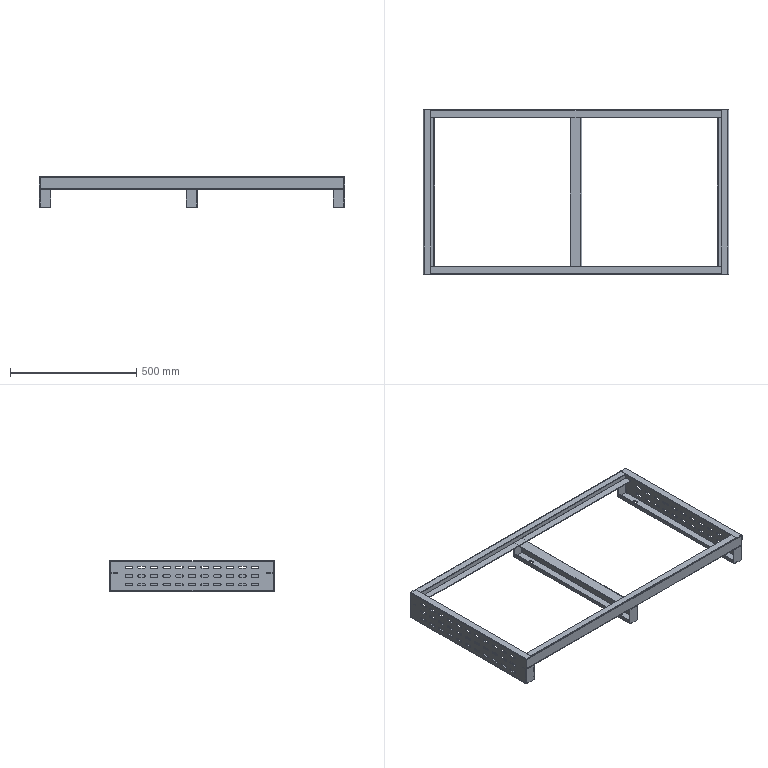Part | SolidWorks | 5 solids | 504 faces | box 1210 x 650 x 120 mm | volume 1821770 mm3 | plane 312 | cylinder 188 | spline 4 | commonest cylinder face diameters 9 x132 0.2 x19 6.2 x19 13 x12 6 x6